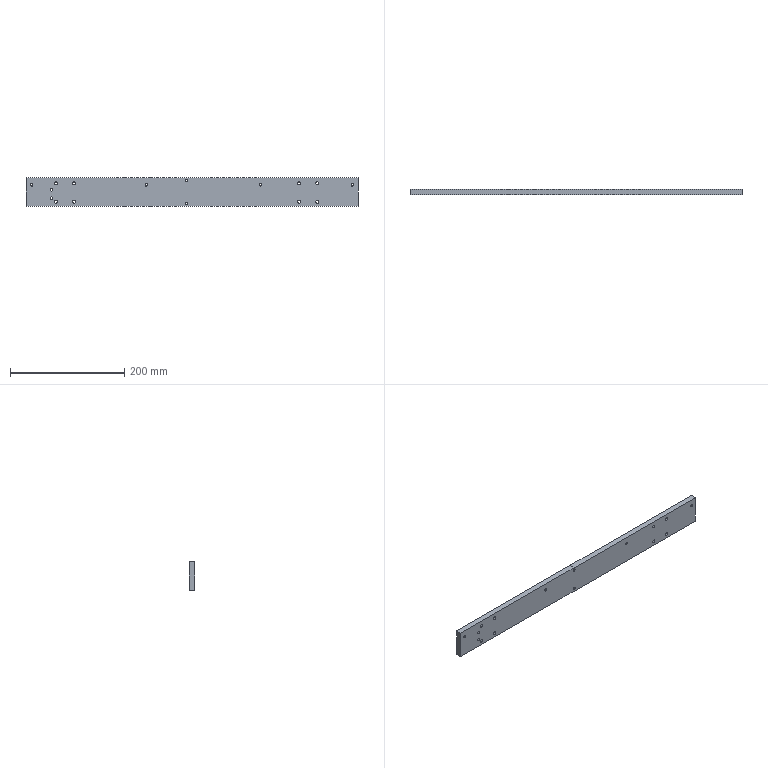Part | STEP file | 0243_223_Plate | 1 solid | 44 faces | box 580 x 10 x 50 mm | volume 286525 mm3 | cylinder 36 | plane 8 | commonest cylinder face diameters 5.5 x16 4.2 x8 4.5 x4 5 x4 8 x4